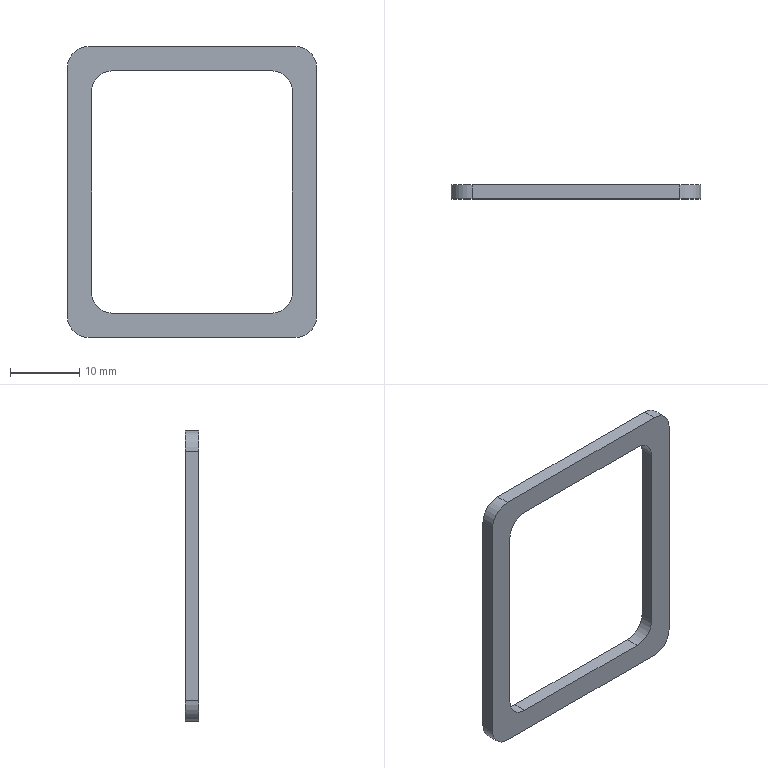Part | STEP file | 10000020458swp000-1 | 1 solid | 18 faces | box 36 x 2 x 42 mm | volume 994 mm3 | plane 10 | cylinder 8 | commonest cylinder face diameters 6 x8
STEP:
#1=CARTESIAN_POINT('',(15.,2.,-21.));
#2=VERTEX_POINT('',#1);
#3=CARTESIAN_POINT('',(-15.,2.,-21.));
#4=VERTEX_POINT('',#3);
#5=CARTESIAN_POINT('',(-18.,2.,-21.));
#6=DIRECTION('',(-1.,0.,0.));
#7=VECTOR('',#6,1000.);
#8=LINE('',#5,#7);
#9=EDGE_CURVE('',#2,#4,#8,.T.);
#10=ORIENTED_EDGE('',*,*,#9,.T.);
#11=CARTESIAN_POINT('',(-18.,2.,-18.));
#12=VERTEX_POINT('',#11);
#13=CARTESIAN_POINT('',(-15.,2.,-18.));
#14=DIRECTION('',(0.,1.,0.));
#15=DIRECTION('',(0.,0.,1.));
#16=AXIS2_PLACEMENT_3D('',#13,#14,#15);
#17=CIRCLE('',#16,3.);
#18=EDGE_CURVE('',#4,#12,#17,.T.);
#19=ORIENTED_EDGE('',*,*,#18,.T.);
#20=CARTESIAN_POINT('',(-18.,2.,18.));
#21=VERTEX_POINT('',#20);
#22=CARTESIAN_POINT('',(-18.,2.,-21.));
#23=DIRECTION('',(0.,0.,1.));
#24=VECTOR('',#23,1000.);
#25=LINE('',#22,#24);
#26=EDGE_CURVE('',#12,#21,#25,.T.);
#27=ORIENTED_EDGE('',*,*,#26,.T.);
#28=CARTESIAN_POINT('',(-15.,2.,21.));
#29=VERTEX_POINT('',#28);
#30=CARTESIAN_POINT('',(-15.,2.,18.));
#31=DIRECTION('',(0.,1.,0.));
#32=DIRECTION('',(0.,0.,1.));
#33=AXIS2_PLACEMENT_3D('',#30,#31,#32);
#34=CIRCLE('',#33,3.);
#35=EDGE_CURVE('',#21,#29,#34,.T.);
#36=ORIENTED_EDGE('',*,*,#35,.T.);
#37=CARTESIAN_POINT('',(15.,2.,21.));
#38=VERTEX_POINT('',#37);
#39=CARTESIAN_POINT('',(-18.,2.,21.));
#40=DIRECTION('',(1.,0.,0.));
#41=VECTOR('',#40,1000.);
#42=LINE('',#39,#41);
#43=EDGE_CURVE('',#29,#38,#42,.T.);
#44=ORIENTED_EDGE('',*,*,#43,.T.);
#45=CARTESIAN_POINT('',(18.,2.,18.));
#46=VERTEX_POINT('',#45);
#47=CARTESIAN_POINT('',(15.,2.,18.));
#48=DIRECTION('',(0.,1.,0.));
#49=DIRECTION('',(0.,0.,1.));
#50=AXIS2_PLACEMENT_3D('',#47,#48,#49);
#51=CIRCLE('',#50,3.);
#52=EDGE_CURVE('',#38,#46,#51,.T.);
#53=ORIENTED_EDGE('',*,*,#52,.T.);
#54=CARTESIAN_POINT('',(18.,2.,-18.));
#55=VERTEX_POINT('',#54);
#56=CARTESIAN_POINT('',(18.,2.,-21.));
#57=DIRECTION('',(0.,0.,-1.));
#58=VECTOR('',#57,1000.);
#59=LINE('',#56,#58);
#60=EDGE_CURVE('',#46,#55,#59,.T.);
#61=ORIENTED_EDGE('',*,*,#60,.T.);
#62=CARTESIAN_POINT('',(15.,2.,-18.));
#63=DIRECTION('',(0.,1.,0.));
#64=DIRECTION('',(0.,0.,1.));
#65=AXIS2_PLACEMENT_3D('',#62,#63,#64);
#66=CIRCLE('',#65,3.);
#67=EDGE_CURVE('',#55,#2,#66,.T.);
#68=ORIENTED_EDGE('',*,*,#67,.T.);
#69=EDGE_LOOP('',(#10,#19,#27,#36,#44,#53,#61,#68));
#70=FACE_OUTER_BOUND('',#69,.T.);
#71=CARTESIAN_POINT('',(-11.5,2.,17.5));
#72=VERTEX_POINT('',#71);
#73=CARTESIAN_POINT('',(11.5,2.,17.5));
#74=VERTEX_POINT('',#73);
#75=CARTESIAN_POINT('',(14.5,2.,17.5));
#76=DIRECTION('',(1.,0.,0.));
#77=VECTOR('',#76,1000.);
#78=LINE('',#75,#77);
#79=EDGE_CURVE('',#72,#74,#78,.T.);
#80=ORIENTED_EDGE('',*,*,#79,.F.);
#81=CARTESIAN_POINT('',(-14.5,2.,14.5));
#82=VERTEX_POINT('',#81);
#83=CARTESIAN_POINT('',(-11.5,2.,14.5));
#84=DIRECTION('',(0.,-1.,0.));
#85=DIRECTION('',(0.,0.,1.));
#86=AXIS2_PLACEMENT_3D('',#83,#84,#85);
#87=CIRCLE('',#86,3.);
#88=EDGE_CURVE('',#72,#82,#87,.T.);
#89=ORIENTED_EDGE('',*,*,#88,.T.);
#90=CARTESIAN_POINT('',(-14.5,2.,-14.5));
#91=VERTEX_POINT('',#90);
#92=CARTESIAN_POINT('',(-14.5,2.,17.5));
#93=DIRECTION('',(0.,0.,1.));
#94=VECTOR('',#93,1000.);
#95=LINE('',#92,#94);
#96=EDGE_CURVE('',#91,#82,#95,.T.);
#97=ORIENTED_EDGE('',*,*,#96,.F.);
#98=CARTESIAN_POINT('',(-11.5,2.,-17.5));
#99=VERTEX_POINT('',#98);
#100=CARTESIAN_POINT('',(-11.5,2.,-14.5));
#101=DIRECTION('',(0.,-1.,0.));
#102=DIRECTION('',(0.,0.,1.));
#103=AXIS2_PLACEMENT_3D('',#100,#101,#102);
#104=CIRCLE('',#103,3.);
#105=EDGE_CURVE('',#91,#99,#104,.T.);
#106=ORIENTED_EDGE('',*,*,#105,.T.);
#107=CARTESIAN_POINT('',(11.5,2.,-17.5));
#108=VERTEX_POINT('',#107);
#109=CARTESIAN_POINT('',(14.5,2.,-17.5));
#110=DIRECTION('',(-1.,0.,0.));
#111=VECTOR('',#110,1000.);
#112=LINE('',#109,#111);
#113=EDGE_CURVE('',#108,#99,#112,.T.);
#114=ORIENTED_EDGE('',*,*,#113,.F.);
#115=CARTESIAN_POINT('',(14.5,2.,-14.5));
#116=VERTEX_POINT('',#115);
#117=CARTESIAN_POINT('',(11.5,2.,-14.5));
#118=DIRECTION('',(0.,-1.,0.));
#119=DIRECTION('',(0.,0.,1.));
#120=AXIS2_PLACEMENT_3D('',#117,#118,#119);
#121=CIRCLE('',#120,3.);
#122=EDGE_CURVE('',#108,#116,#121,.T.);
#123=ORIENTED_EDGE('',*,*,#122,.T.);
#124=CARTESIAN_POINT('',(14.5,2.,14.5));
#125=VERTEX_POINT('',#124);
#126=CARTESIAN_POINT('',(14.5,2.,17.5));
#127=DIRECTION('',(0.,0.,-1.));
#128=VECTOR('',#127,1000.);
#129=LINE('',#126,#128);
#130=EDGE_CURVE('',#125,#116,#129,.T.);
#131=ORIENTED_EDGE('',*,*,#130,.F.);
#132=CARTESIAN_POINT('',(11.5,2.,14.5));
#133=DIRECTION('',(0.,-1.,0.));
#134=DIRECTION('',(0.,0.,1.));
#135=AXIS2_PLACEMENT_3D('',#132,#133,#134);
#136=CIRCLE('',#135,3.);
#137=EDGE_CURVE('',#125,#74,#136,.T.);
#138=ORIENTED_EDGE('',*,*,#137,.T.);
#139=EDGE_LOOP('',(#80,#89,#97,#106,#114,#123,#131,#138));
#140=FACE_BOUND('',#139,.T.);
#141=CARTESIAN_POINT('',(0.,2.,0.));
#142=DIRECTION('',(0.,1.,0.));
#143=DIRECTION('',(0.,0.,1.));
#144=AXIS2_PLACEMENT_3D('',#141,#142,#143);
#145=PLANE('',#144);
#146=ADVANCED_FACE('',(#70,#140),#145,.T.);
#147=CARTESIAN_POINT('',(-18.,0.,-18.));
#148=VERTEX_POINT('',#147);
#149=CARTESIAN_POINT('',(-18.,0.,18.));
#150=VERTEX_POINT('',#149);
#151=CARTESIAN_POINT('',(-18.,0.,-21.));
#152=DIRECTION('',(0.,0.,1.));
#153=VECTOR('',#152,1000.);
#154=LINE('',#151,#153);
#155=EDGE_CURVE('',#148,#150,#154,.T.);
#156=ORIENTED_EDGE('',*,*,#155,.F.);
#157=CARTESIAN_POINT('',(-15.,0.,-21.));
#158=VERTEX_POINT('',#157);
#159=CARTESIAN_POINT('',(-15.,0.,-18.));
#160=DIRECTION('',(0.,-1.,0.));
#161=DIRECTION('',(0.,0.,1.));
#162=AXIS2_PLACEMENT_3D('',#159,#160,#161);
#163=CIRCLE('',#162,3.);
#164=EDGE_CURVE('',#148,#158,#163,.T.);
#165=ORIENTED_EDGE('',*,*,#164,.T.);
#166=CARTESIAN_POINT('',(15.,0.,-21.));
#167=VERTEX_POINT('',#166);
#168=CARTESIAN_POINT('',(-18.,0.,-21.));
#169=DIRECTION('',(-1.,0.,0.));
#170=VECTOR('',#169,1000.);
#171=LINE('',#168,#170);
#172=EDGE_CURVE('',#167,#158,#171,.T.);
#173=ORIENTED_EDGE('',*,*,#172,.F.);
#174=CARTESIAN_POINT('',(18.,0.,-18.));
#175=VERTEX_POINT('',#174);
#176=CARTESIAN_POINT('',(15.,0.,-18.));
#177=DIRECTION('',(0.,-1.,0.));
#178=DIRECTION('',(0.,0.,1.));
#179=AXIS2_PLACEMENT_3D('',#176,#177,#178);
#180=CIRCLE('',#179,3.);
#181=EDGE_CURVE('',#167,#175,#180,.T.);
#182=ORIENTED_EDGE('',*,*,#181,.T.);
#183=CARTESIAN_POINT('',(18.,0.,18.));
#184=VERTEX_POINT('',#183);
#185=CARTESIAN_POINT('',(18.,0.,-21.));
#186=DIRECTION('',(0.,0.,-1.));
#187=VECTOR('',#186,1000.);
#188=LINE('',#185,#187);
#189=EDGE_CURVE('',#184,#175,#188,.T.);
#190=ORIENTED_EDGE('',*,*,#189,.F.);
#191=CARTESIAN_POINT('',(15.,0.,21.));
#192=VERTEX_POINT('',#191);
#193=CARTESIAN_POINT('',(15.,0.,18.));
#194=DIRECTION('',(0.,-1.,0.));
#195=DIRECTION('',(0.,0.,1.));
#196=AXIS2_PLACEMENT_3D('',#193,#194,#195);
#197=CIRCLE('',#196,3.);
#198=EDGE_CURVE('',#184,#192,#197,.T.);
#199=ORIENTED_EDGE('',*,*,#198,.T.);
#200=CARTESIAN_POINT('',(-15.,0.,21.));
#201=VERTEX_POINT('',#200);
#202=CARTESIAN_POINT('',(-18.,0.,21.));
#203=DIRECTION('',(1.,0.,0.));
#204=VECTOR('',#203,1000.);
#205=LINE('',#202,#204);
#206=EDGE_CURVE('',#201,#192,#205,.T.);
#207=ORIENTED_EDGE('',*,*,#206,.F.);
#208=CARTESIAN_POINT('',(-15.,0.,18.));
#209=DIRECTION('',(0.,-1.,0.));
#210=DIRECTION('',(0.,0.,1.));
#211=AXIS2_PLACEMENT_3D('',#208,#209,#210);
#212=CIRCLE('',#211,3.);
#213=EDGE_CURVE('',#201,#150,#212,.T.);
#214=ORIENTED_EDGE('',*,*,#213,.T.);
#215=EDGE_LOOP('',(#156,#165,#173,#182,#190,#199,#207,#214));
#216=FACE_OUTER_BOUND('',#215,.T.);
#217=CARTESIAN_POINT('',(11.5,0.,-17.5));
#218=VERTEX_POINT('',#217);
#219=CARTESIAN_POINT('',(-11.5,0.,-17.5));
#220=VERTEX_POINT('',#219);
#221=CARTESIAN_POINT('',(14.5,0.,-17.5));
#222=DIRECTION('',(-1.,0.,0.));
#223=VECTOR('',#222,1000.);
#224=LINE('',#221,#223);
#225=EDGE_CURVE('',#218,#220,#224,.T.);
#226=ORIENTED_EDGE('',*,*,#225,.T.);
#227=CARTESIAN_POINT('',(-14.5,0.,-14.5));
#228=VERTEX_POINT('',#227);
#229=CARTESIAN_POINT('',(-11.5,0.,-14.5));
#230=DIRECTION('',(0.,1.,0.));
#231=DIRECTION('',(0.,0.,1.));
#232=AXIS2_PLACEMENT_3D('',#229,#230,#231);
#233=CIRCLE('',#232,3.);
#234=EDGE_CURVE('',#220,#228,#233,.T.);
#235=ORIENTED_EDGE('',*,*,#234,.T.);
#236=CARTESIAN_POINT('',(-14.5,0.,14.5));
#237=VERTEX_POINT('',#236);
#238=CARTESIAN_POINT('',(-14.5,0.,17.5));
#239=DIRECTION('',(0.,0.,1.));
#240=VECTOR('',#239,1000.);
#241=LINE('',#238,#240);
#242=EDGE_CURVE('',#228,#237,#241,.T.);
#243=ORIENTED_EDGE('',*,*,#242,.T.);
#244=CARTESIAN_POINT('',(-11.5,0.,17.5));
#245=VERTEX_POINT('',#244);
#246=CARTESIAN_POINT('',(-11.5,0.,14.5));
#247=DIRECTION('',(0.,1.,0.));
#248=DIRECTION('',(0.,0.,1.));
#249=AXIS2_PLACEMENT_3D('',#246,#247,#248);
#250=CIRCLE('',#249,3.);
#251=EDGE_CURVE('',#237,#245,#250,.T.);
#252=ORIENTED_EDGE('',*,*,#251,.T.);
#253=CARTESIAN_POINT('',(11.5,0.,17.5));
#254=VERTEX_POINT('',#253);
#255=CARTESIAN_POINT('',(14.5,0.,17.5));
#256=DIRECTION('',(1.,0.,0.));
#257=VECTOR('',#256,1000.);
#258=LINE('',#255,#257);
#259=EDGE_CURVE('',#245,#254,#258,.T.);
#260=ORIENTED_EDGE('',*,*,#259,.T.);
#261=CARTESIAN_POINT('',(14.5,0.,14.5));
#262=VERTEX_POINT('',#261);
#263=CARTESIAN_POINT('',(11.5,0.,14.5));
#264=DIRECTION('',(0.,1.,0.));
#265=DIRECTION('',(0.,0.,1.));
#266=AXIS2_PLACEMENT_3D('',#263,#264,#265);
#267=CIRCLE('',#266,3.);
#268=EDGE_CURVE('',#254,#262,#267,.T.);
#269=ORIENTED_EDGE('',*,*,#268,.T.);
#270=CARTESIAN_POINT('',(14.5,0.,-14.5));
#271=VERTEX_POINT('',#270);
#272=CARTESIAN_POINT('',(14.5,0.,17.5));
#273=DIRECTION('',(0.,0.,-1.));
#274=VECTOR('',#273,1000.);
#275=LINE('',#272,#274);
#276=EDGE_CURVE('',#262,#271,#275,.T.);
#277=ORIENTED_EDGE('',*,*,#276,.T.);
#278=CARTESIAN_POINT('',(11.5,0.,-14.5));
#279=DIRECTION('',(0.,1.,0.));
#280=DIRECTION('',(0.,0.,1.));
#281=AXIS2_PLACEMENT_3D('',#278,#279,#280);
#282=CIRCLE('',#281,3.);
#283=EDGE_CURVE('',#271,#218,#282,.T.);
#284=ORIENTED_EDGE('',*,*,#283,.T.);
#285=EDGE_LOOP('',(#226,#235,#243,#252,#260,#269,#277,#284));
#286=FACE_BOUND('',#285,.T.);
#287=CARTESIAN_POINT('',(0.,0.,0.));
#288=DIRECTION('',(0.,1.,0.));
#289=DIRECTION('',(0.,0.,1.));
#290=AXIS2_PLACEMENT_3D('',#287,#288,#289);
#291=PLANE('',#290);
#292=ADVANCED_FACE('',(#216,#286),#291,.F.);
#293=ORIENTED_EDGE('',*,*,#189,.T.);
#294=CARTESIAN_POINT('',(18.,2.,-18.));
#295=DIRECTION('',(0.,1.,0.));
#296=VECTOR('',#295,1000.);
#297=LINE('',#294,#296);
#298=EDGE_CURVE('',#175,#55,#297,.T.);
#299=ORIENTED_EDGE('',*,*,#298,.T.);
#300=ORIENTED_EDGE('',*,*,#60,.F.);
#301=CARTESIAN_POINT('',(18.,2.,18.));
#302=DIRECTION('',(0.,-1.,0.));
#303=VECTOR('',#302,1000.);
#304=LINE('',#301,#303);
#305=EDGE_CURVE('',#46,#184,#304,.T.);
#306=ORIENTED_EDGE('',*,*,#305,.T.);
#307=EDGE_LOOP('',(#293,#299,#300,#306));
#308=FACE_OUTER_BOUND('',#307,.T.);
#309=CARTESIAN_POINT('',(18.,2.,-21.));
#310=DIRECTION('',(-1.,0.,0.));
#311=DIRECTION('',(0.,0.,1.));
#312=AXIS2_PLACEMENT_3D('',#309,#310,#311);
#313=PLANE('',#312);
#314=ADVANCED_FACE('',(#308),#313,.F.);
#315=ORIENTED_EDGE('',*,*,#172,.T.);
#316=CARTESIAN_POINT('',(-15.,2.,-21.));
#317=DIRECTION('',(0.,1.,0.));
#318=VECTOR('',#317,1000.);
#319=LINE('',#316,#318);
#320=EDGE_CURVE('',#158,#4,#319,.T.);
#321=ORIENTED_EDGE('',*,*,#320,.T.);
#322=ORIENTED_EDGE('',*,*,#9,.F.);
#323=CARTESIAN_POINT('',(15.,2.,-21.));
#324=DIRECTION('',(0.,-1.,0.));
#325=VECTOR('',#324,1000.);
#326=LINE('',#323,#325);
#327=EDGE_CURVE('',#2,#167,#326,.T.);
#328=ORIENTED_EDGE('',*,*,#327,.T.);
#329=EDGE_LOOP('',(#315,#321,#322,#328));
#330=FACE_OUTER_BOUND('',#329,.T.);
#331=CARTESIAN_POINT('',(-18.,2.,-21.));
#332=DIRECTION('',(0.,0.,1.));
#333=DIRECTION('',(1.,0.,0.));
#334=AXIS2_PLACEMENT_3D('',#331,#332,#333);
#335=PLANE('',#334);
#336=ADVANCED_FACE('',(#330),#335,.F.);
#337=ORIENTED_EDGE('',*,*,#26,.F.);
#338=CARTESIAN_POINT('',(-18.,2.,-18.));
#339=DIRECTION('',(0.,-1.,0.));
#340=VECTOR('',#339,1000.);
#341=LINE('',#338,#340);
#342=EDGE_CURVE('',#12,#148,#341,.T.);
#343=ORIENTED_EDGE('',*,*,#342,.T.);
#344=ORIENTED_EDGE('',*,*,#155,.T.);
#345=CARTESIAN_POINT('',(-18.,2.,18.));
#346=DIRECTION('',(0.,1.,0.));
#347=VECTOR('',#346,1000.);
#348=LINE('',#345,#347);
#349=EDGE_CURVE('',#150,#21,#348,.T.);
#350=ORIENTED_EDGE('',*,*,#349,.T.);
#351=EDGE_LOOP('',(#337,#343,#344,#350));
#352=FACE_OUTER_BOUND('',#351,.T.);
#353=CARTESIAN_POINT('',(-18.,2.,-21.));
#354=DIRECTION('',(1.,0.,0.));
#355=DIRECTION('',(0.,0.,-1.));
#356=AXIS2_PLACEMENT_3D('',#353,#354,#355);
#357=PLANE('',#356);
#358=ADVANCED_FACE('',(#352),#357,.F.);
#359=ORIENTED_EDGE('',*,*,#206,.T.);
#360=CARTESIAN_POINT('',(15.,2.,21.));
#361=DIRECTION('',(0.,1.,0.));
#362=VECTOR('',#361,1000.);
#363=LINE('',#360,#362);
#364=EDGE_CURVE('',#192,#38,#363,.T.);
#365=ORIENTED_EDGE('',*,*,#364,.T.);
#366=ORIENTED_EDGE('',*,*,#43,.F.);
#367=CARTESIAN_POINT('',(-15.,2.,21.));
#368=DIRECTION('',(0.,-1.,0.));
#369=VECTOR('',#368,1000.);
#370=LINE('',#367,#369);
#371=EDGE_CURVE('',#29,#201,#370,.T.);
#372=ORIENTED_EDGE('',*,*,#371,.T.);
#373=EDGE_LOOP('',(#359,#365,#366,#372));
#374=FACE_OUTER_BOUND('',#373,.T.);
#375=CARTESIAN_POINT('',(-18.,2.,21.));
#376=DIRECTION('',(0.,0.,-1.));
#377=DIRECTION('',(-1.,0.,0.));
#378=AXIS2_PLACEMENT_3D('',#375,#376,#377);
#379=PLANE('',#378);
#380=ADVANCED_FACE('',(#374),#379,.F.);
#381=ORIENTED_EDGE('',*,*,#96,.T.);
#382=CARTESIAN_POINT('',(-14.5,0.,14.5));
#383=DIRECTION('',(0.,-1.,0.));
#384=VECTOR('',#383,1000.);
#385=LINE('',#382,#384);
#386=EDGE_CURVE('',#82,#237,#385,.T.);
#387=ORIENTED_EDGE('',*,*,#386,.T.);
#388=ORIENTED_EDGE('',*,*,#242,.F.);
#389=CARTESIAN_POINT('',(-14.5,2.,-14.5));
#390=DIRECTION('',(0.,1.,0.));
#391=VECTOR('',#390,1000.);
#392=LINE('',#389,#391);
#393=EDGE_CURVE('',#228,#91,#392,.T.);
#394=ORIENTED_EDGE('',*,*,#393,.T.);
#395=EDGE_LOOP('',(#381,#387,#388,#394));
#396=FACE_OUTER_BOUND('',#395,.T.);
#397=CARTESIAN_POINT('',(-14.5,2.,17.5));
#398=DIRECTION('',(1.,0.,0.));
#399=DIRECTION('',(0.,0.,-1.));
#400=AXIS2_PLACEMENT_3D('',#397,#398,#399);
#401=PLANE('',#400);
#402=ADVANCED_FACE('',(#396),#401,.T.);
#403=ORIENTED_EDGE('',*,*,#259,.F.);
#404=CARTESIAN_POINT('',(-11.5,2.,17.5));
#405=DIRECTION('',(0.,1.,0.));
#406=VECTOR('',#405,1000.);
#407=LINE('',#404,#406);
#408=EDGE_CURVE('',#245,#72,#407,.T.);
#409=ORIENTED_EDGE('',*,*,#408,.T.);
#410=ORIENTED_EDGE('',*,*,#79,.T.);
#411=CARTESIAN_POINT('',(11.5,0.,17.5));
#412=DIRECTION('',(0.,-1.,0.));
#413=VECTOR('',#412,1000.);
#414=LINE('',#411,#413);
#415=EDGE_CURVE('',#74,#254,#414,.T.);
#416=ORIENTED_EDGE('',*,*,#415,.T.);
#417=EDGE_LOOP('',(#403,#409,#410,#416));
#418=FACE_OUTER_BOUND('',#417,.T.);
#419=CARTESIAN_POINT('',(14.5,2.,17.5));
#420=DIRECTION('',(0.,0.,-1.));
#421=DIRECTION('',(-1.,0.,0.));
#422=AXIS2_PLACEMENT_3D('',#419,#420,#421);
#423=PLANE('',#422);
#424=ADVANCED_FACE('',(#418),#423,.T.);
#425=ORIENTED_EDGE('',*,*,#276,.F.);
#426=CARTESIAN_POINT('',(14.5,2.,14.5));
#427=DIRECTION('',(0.,1.,0.));
#428=VECTOR('',#427,1000.);
#429=LINE('',#426,#428);
#430=EDGE_CURVE('',#262,#125,#429,.T.);
#431=ORIENTED_EDGE('',*,*,#430,.T.);
#432=ORIENTED_EDGE('',*,*,#130,.T.);
#433=CARTESIAN_POINT('',(14.5,0.,-14.5));
#434=DIRECTION('',(0.,-1.,0.));
#435=VECTOR('',#434,1000.);
#436=LINE('',#433,#435);
#437=EDGE_CURVE('',#116,#271,#436,.T.);
#438=ORIENTED_EDGE('',*,*,#437,.T.);
#439=EDGE_LOOP('',(#425,#431,#432,#438));
#440=FACE_OUTER_BOUND('',#439,.T.);
#441=CARTESIAN_POINT('',(14.5,2.,17.5));
#442=DIRECTION('',(-1.,0.,0.));
#443=DIRECTION('',(0.,0.,1.));
#444=AXIS2_PLACEMENT_3D('',#441,#442,#443);
#445=PLANE('',#444);
#446=ADVANCED_FACE('',(#440),#445,.T.);
#447=ORIENTED_EDGE('',*,*,#225,.F.);
#448=CARTESIAN_POINT('',(11.5,2.,-17.5));
#449=DIRECTION('',(0.,1.,0.));
#450=VECTOR('',#449,1000.);
#451=LINE('',#448,#450);
#452=EDGE_CURVE('',#218,#108,#451,.T.);
#453=ORIENTED_EDGE('',*,*,#452,.T.);
#454=ORIENTED_EDGE('',*,*,#113,.T.);
#455=CARTESIAN_POINT('',(-11.5,0.,-17.5));
#456=DIRECTION('',(0.,-1.,0.));
#457=VECTOR('',#456,1000.);
#458=LINE('',#455,#457);
#459=EDGE_CURVE('',#99,#220,#458,.T.);
#460=ORIENTED_EDGE('',*,*,#459,.T.);
#461=EDGE_LOOP('',(#447,#453,#454,#460));
#462=FACE_OUTER_BOUND('',#461,.T.);
#463=CARTESIAN_POINT('',(14.5,2.,-17.5));
#464=DIRECTION('',(0.,0.,1.));
#465=DIRECTION('',(1.,0.,0.));
#466=AXIS2_PLACEMENT_3D('',#463,#464,#465);
#467=PLANE('',#466);
#468=ADVANCED_FACE('',(#462),#467,.T.);
#469=ORIENTED_EDGE('',*,*,#88,.F.);
#470=ORIENTED_EDGE('',*,*,#408,.F.);
#471=ORIENTED_EDGE('',*,*,#251,.F.);
#472=ORIENTED_EDGE('',*,*,#386,.F.);
#473=EDGE_LOOP('',(#469,#470,#471,#472));
#474=FACE_OUTER_BOUND('',#473,.T.);
#475=CARTESIAN_POINT('',(-11.5,2.,14.5));
#476=DIRECTION('',(0.,1.,0.));
#477=DIRECTION('',(0.,0.,1.));
#478=AXIS2_PLACEMENT_3D('',#475,#476,#477);
#479=CYLINDRICAL_SURFACE('',#478,3.);
#480=ADVANCED_FACE('',(#474),#479,.F.);
#481=ORIENTED_EDGE('',*,*,#137,.F.);
#482=ORIENTED_EDGE('',*,*,#430,.F.);
#483=ORIENTED_EDGE('',*,*,#268,.F.);
#484=ORIENTED_EDGE('',*,*,#415,.F.);
#485=EDGE_LOOP('',(#481,#482,#483,#484));
#486=FACE_OUTER_BOUND('',#485,.T.);
#487=CARTESIAN_POINT('',(11.5,2.,14.5));
#488=DIRECTION('',(0.,1.,0.));
#489=DIRECTION('',(0.,0.,1.));
#490=AXIS2_PLACEMENT_3D('',#487,#488,#489);
#491=CYLINDRICAL_SURFACE('',#490,3.);
#492=ADVANCED_FACE('',(#486),#491,.F.);
#493=ORIENTED_EDGE('',*,*,#122,.F.);
#494=ORIENTED_EDGE('',*,*,#452,.F.);
#495=ORIENTED_EDGE('',*,*,#283,.F.);
#496=ORIENTED_EDGE('',*,*,#437,.F.);
#497=EDGE_LOOP('',(#493,#494,#495,#496));
#498=FACE_OUTER_BOUND('',#497,.T.);
#499=CARTESIAN_POINT('',(11.5,2.,-14.5));
#500=DIRECTION('',(0.,1.,0.));
#501=DIRECTION('',(0.,0.,1.));
#502=AXIS2_PLACEMENT_3D('',#499,#500,#501);
#503=CYLINDRICAL_SURFACE('',#502,3.);
#504=ADVANCED_FACE('',(#498),#503,.F.);
#505=ORIENTED_EDGE('',*,*,#18,.F.);
#506=ORIENTED_EDGE('',*,*,#320,.F.);
#507=ORIENTED_EDGE('',*,*,#164,.F.);
#508=ORIENTED_EDGE('',*,*,#342,.F.);
#509=EDGE_LOOP('',(#505,#506,#507,#508));
#510=FACE_OUTER_BOUND('',#509,.T.);
#511=CARTESIAN_POINT('',(-15.,2.,-18.));
#512=DIRECTION('',(0.,-1.,0.));
#513=DIRECTION('',(0.,0.,-1.));
#514=AXIS2_PLACEMENT_3D('',#511,#512,#513);
#515=CYLINDRICAL_SURFACE('',#514,3.);
#516=ADVANCED_FACE('',(#510),#515,.T.);
#517=ORIENTED_EDGE('',*,*,#105,.F.);
#518=ORIENTED_EDGE('',*,*,#393,.F.);
#519=ORIENTED_EDGE('',*,*,#234,.F.);
#520=ORIENTED_EDGE('',*,*,#459,.F.);
#521=EDGE_LOOP('',(#517,#518,#519,#520));
#522=FACE_OUTER_BOUND('',#521,.T.);
#523=CARTESIAN_POINT('',(-11.5,2.,-14.5));
#524=DIRECTION('',(0.,1.,0.));
#525=DIRECTION('',(0.,0.,1.));
#526=AXIS2_PLACEMENT_3D('',#523,#524,#525);
#527=CYLINDRICAL_SURFACE('',#526,3.);
#528=ADVANCED_FACE('',(#522),#527,.F.);
#529=ORIENTED_EDGE('',*,*,#67,.F.);
#530=ORIENTED_EDGE('',*,*,#298,.F.);
#531=ORIENTED_EDGE('',*,*,#181,.F.);
#532=ORIENTED_EDGE('',*,*,#327,.F.);
#533=EDGE_LOOP('',(#529,#530,#531,#532));
#534=FACE_OUTER_BOUND('',#533,.T.);
#535=CARTESIAN_POINT('',(15.,2.,-18.));
#536=DIRECTION('',(0.,-1.,0.));
#537=DIRECTION('',(0.,0.,-1.));
#538=AXIS2_PLACEMENT_3D('',#535,#536,#537);
#539=CYLINDRICAL_SURFACE('',#538,3.);
#540=ADVANCED_FACE('',(#534),#539,.T.);
#541=ORIENTED_EDGE('',*,*,#52,.F.);
#542=ORIENTED_EDGE('',*,*,#364,.F.);
#543=ORIENTED_EDGE('',*,*,#198,.F.);
#544=ORIENTED_EDGE('',*,*,#305,.F.);
#545=EDGE_LOOP('',(#541,#542,#543,#544));
#546=FACE_OUTER_BOUND('',#545,.T.);
#547=CARTESIAN_POINT('',(15.,2.,18.));
#548=DIRECTION('',(0.,-1.,0.));
#549=DIRECTION('',(0.,0.,-1.));
#550=AXIS2_PLACEMENT_3D('',#547,#548,#549);
#551=CYLINDRICAL_SURFACE('',#550,3.);
#552=ADVANCED_FACE('',(#546),#551,.T.);
#553=ORIENTED_EDGE('',*,*,#35,.F.);
#554=ORIENTED_EDGE('',*,*,#349,.F.);
#555=ORIENTED_EDGE('',*,*,#213,.F.);
#556=ORIENTED_EDGE('',*,*,#371,.F.);
#557=EDGE_LOOP('',(#553,#554,#555,#556));
#558=FACE_OUTER_BOUND('',#557,.T.);
#559=CARTESIAN_POINT('',(-15.,2.,18.));
#560=DIRECTION('',(0.,-1.,0.));
#561=DIRECTION('',(0.,0.,-1.));
#562=AXIS2_PLACEMENT_3D('',#559,#560,#561);
#563=CYLINDRICAL_SURFACE('',#562,3.);
#564=ADVANCED_FACE('',(#558),#563,.T.);
#565=CLOSED_SHELL('',(#146,#292,#314,#336,#358,#380,#402,#424,#446,#468,#480,#492,#504,#516,#528,#540,#552,#564));
#566=MANIFOLD_SOLID_BREP('',#565);
#567=CARTESIAN_POINT('',(0.,0.,0.));
#568=DIRECTION('',(0.,0.,1.));
#569=DIRECTION('',(1.,0.,0.));
#570=AXIS2_PLACEMENT_3D('',#567,#568,#569);
#571=(LENGTH_UNIT()NAMED_UNIT(*)SI_UNIT(.MILLI.,.METRE.));
#572=UNCERTAINTY_MEASURE_WITH_UNIT(LENGTH_MEASURE(0.00001),#571,'','');
#573=(NAMED_UNIT(*)PLANE_ANGLE_UNIT()SI_UNIT($,.RADIAN.));
#574=(NAMED_UNIT(*)SI_UNIT($,.STERADIAN.)SOLID_ANGLE_UNIT());
#575=(GEOMETRIC_REPRESENTATION_CONTEXT(3)GLOBAL_UNCERTAINTY_ASSIGNED_CONTEXT((#572))GLOBAL_UNIT_ASSIGNED_CONTEXT((#571,#573,#574))REPRESENTATION_CONTEXT('',''));
#576=ADVANCED_BREP_SHAPE_REPRESENTATION('',(#566,#570),#575);